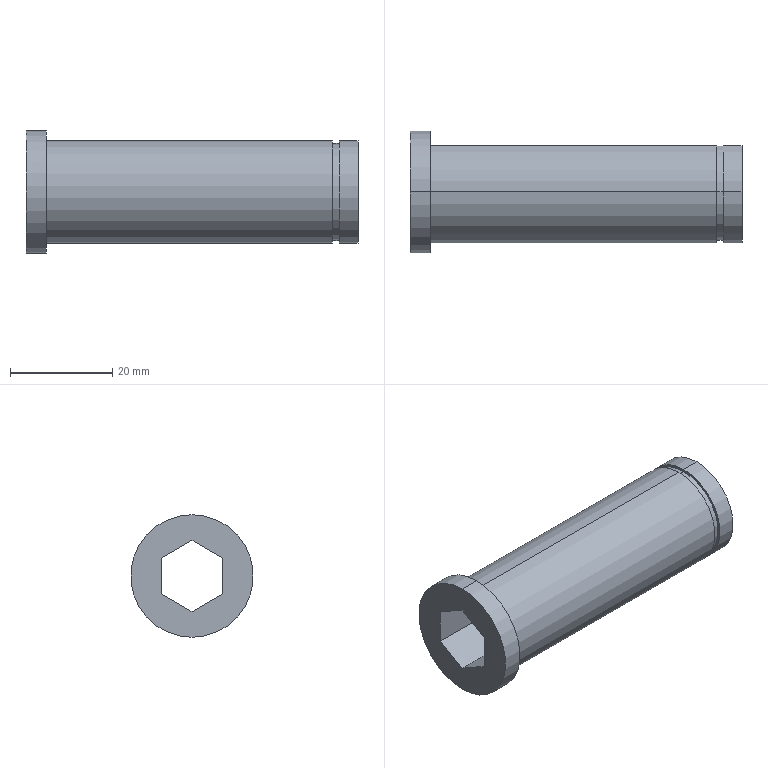Part | SolidWorks | features BaseBody 1 | 1 solid | 23 faces | box 65 x 24 x 24 mm | volume 12337 mm3 | plane 12 | cylinder 11 | commonest cylinder face diameters 20 x6 19 x3 24 x2
STEP:
#1=CARTESIAN_POINT('',(60.,9.,3.041));
#2=VERTEX_POINT('',#1);
#3=CARTESIAN_POINT('',(60.,0.,9.5));
#4=VERTEX_POINT('',#3);
#5=CARTESIAN_POINT('',(60.,0.,0.));
#6=DIRECTION('',(1.,0.,0.));
#7=DIRECTION('',(0.,0.,-1.));
#8=AXIS2_PLACEMENT_3D('',#5,#6,#7);
#9=CIRCLE('',#8,9.5);
#10=EDGE_CURVE('',#2,#4,#9,.T.);
#11=ORIENTED_EDGE('',*,*,#10,.T.);
#12=CARTESIAN_POINT('',(61.35,0.,9.5));
#13=VERTEX_POINT('',#12);
#14=CARTESIAN_POINT('',(65.,0.,9.5));
#15=DIRECTION('',(1.,0.,0.));
#16=VECTOR('',#15,1000.);
#17=LINE('',#14,#16);
#18=EDGE_CURVE('',#4,#13,#17,.T.);
#19=ORIENTED_EDGE('',*,*,#18,.T.);
#20=CARTESIAN_POINT('',(61.35,9.,3.041));
#21=VERTEX_POINT('',#20);
#22=CARTESIAN_POINT('',(61.35,0.,0.));
#23=DIRECTION('',(1.,0.,0.));
#24=DIRECTION('',(0.,0.,-1.));
#25=AXIS2_PLACEMENT_3D('',#22,#23,#24);
#26=CIRCLE('',#25,9.5);
#27=EDGE_CURVE('',#21,#13,#26,.T.);
#28=ORIENTED_EDGE('',*,*,#27,.F.);
#29=CARTESIAN_POINT('',(65.,9.,3.041));
#30=DIRECTION('',(-1.,0.,0.));
#31=VECTOR('',#30,1000.);
#32=LINE('',#29,#31);
#33=EDGE_CURVE('',#21,#2,#32,.T.);
#34=ORIENTED_EDGE('',*,*,#33,.T.);
#35=EDGE_LOOP('',(#11,#19,#28,#34));
#36=FACE_OUTER_BOUND('',#35,.T.);
#37=CARTESIAN_POINT('',(65.,0.,0.));
#38=DIRECTION('',(1.,0.,0.));
#39=DIRECTION('',(0.,0.,-1.));
#40=AXIS2_PLACEMENT_3D('',#37,#38,#39);
#41=CYLINDRICAL_SURFACE('',#40,9.5);
#42=ADVANCED_FACE('',(#36),#41,.T.);
#43=ORIENTED_EDGE('',*,*,#18,.F.);
#44=CARTESIAN_POINT('',(60.,0.,-9.5));
#45=VERTEX_POINT('',#44);
#46=CARTESIAN_POINT('',(60.,0.,0.));
#47=DIRECTION('',(1.,0.,0.));
#48=DIRECTION('',(0.,0.,-1.));
#49=AXIS2_PLACEMENT_3D('',#46,#47,#48);
#50=CIRCLE('',#49,9.5);
#51=EDGE_CURVE('',#4,#45,#50,.T.);
#52=ORIENTED_EDGE('',*,*,#51,.T.);
#53=CARTESIAN_POINT('',(61.35,0.,-9.5));
#54=VERTEX_POINT('',#53);
#55=CARTESIAN_POINT('',(65.,0.,-9.5));
#56=DIRECTION('',(1.,0.,0.));
#57=VECTOR('',#56,1000.);
#58=LINE('',#55,#57);
#59=EDGE_CURVE('',#45,#54,#58,.T.);
#60=ORIENTED_EDGE('',*,*,#59,.T.);
#61=CARTESIAN_POINT('',(61.35,0.,0.));
#62=DIRECTION('',(1.,0.,0.));
#63=DIRECTION('',(0.,0.,-1.));
#64=AXIS2_PLACEMENT_3D('',#61,#62,#63);
#65=CIRCLE('',#64,9.5);
#66=EDGE_CURVE('',#13,#54,#65,.T.);
#67=ORIENTED_EDGE('',*,*,#66,.F.);
#68=EDGE_LOOP('',(#43,#52,#60,#67));
#69=FACE_OUTER_BOUND('',#68,.T.);
#70=CARTESIAN_POINT('',(65.,0.,0.));
#71=DIRECTION('',(1.,0.,0.));
#72=DIRECTION('',(0.,0.,-1.));
#73=AXIS2_PLACEMENT_3D('',#70,#71,#72);
#74=CYLINDRICAL_SURFACE('',#73,9.5);
#75=ADVANCED_FACE('',(#69),#74,.T.);
#76=CARTESIAN_POINT('',(65.,0.,-10.));
#77=VERTEX_POINT('',#76);
#78=CARTESIAN_POINT('',(65.,9.,-4.359));
#79=VERTEX_POINT('',#78);
#80=CARTESIAN_POINT('',(65.,0.,0.));
#81=DIRECTION('',(1.,0.,0.));
#82=DIRECTION('',(0.,0.,-1.));
#83=AXIS2_PLACEMENT_3D('',#80,#81,#82);
#84=CIRCLE('',#83,10.);
#85=EDGE_CURVE('',#77,#79,#84,.T.);
#86=ORIENTED_EDGE('',*,*,#85,.F.);
#87=CARTESIAN_POINT('',(61.35,0.,-10.));
#88=VERTEX_POINT('',#87);
#89=CARTESIAN_POINT('',(77.,0.,-10.));
#90=DIRECTION('',(-1.,0.,0.));
#91=VECTOR('',#90,1000.);
#92=LINE('',#89,#91);
#93=EDGE_CURVE('',#77,#88,#92,.T.);
#94=ORIENTED_EDGE('',*,*,#93,.T.);
#95=CARTESIAN_POINT('',(61.35,9.,-4.359));
#96=VERTEX_POINT('',#95);
#97=CARTESIAN_POINT('',(61.35,0.,0.));
#98=DIRECTION('',(1.,0.,0.));
#99=DIRECTION('',(0.,0.,-1.));
#100=AXIS2_PLACEMENT_3D('',#97,#98,#99);
#101=CIRCLE('',#100,10.);
#102=EDGE_CURVE('',#88,#96,#101,.T.);
#103=ORIENTED_EDGE('',*,*,#102,.T.);
#104=CARTESIAN_POINT('',(77.,9.,-4.359));
#105=DIRECTION('',(1.,0.,0.));
#106=VECTOR('',#105,1000.);
#107=LINE('',#104,#106);
#108=EDGE_CURVE('',#96,#79,#107,.T.);
#109=ORIENTED_EDGE('',*,*,#108,.T.);
#110=EDGE_LOOP('',(#86,#94,#103,#109));
#111=FACE_OUTER_BOUND('',#110,.T.);
#112=CARTESIAN_POINT('',(77.,0.,0.));
#113=DIRECTION('',(-1.,0.,0.));
#114=DIRECTION('',(0.,0.,1.));
#115=AXIS2_PLACEMENT_3D('',#112,#113,#114);
#116=CYLINDRICAL_SURFACE('',#115,10.);
#117=ADVANCED_FACE('',(#111),#116,.T.);
#118=ORIENTED_EDGE('',*,*,#93,.F.);
#119=CARTESIAN_POINT('',(65.,0.,10.));
#120=VERTEX_POINT('',#119);
#121=CARTESIAN_POINT('',(65.,0.,0.));
#122=DIRECTION('',(1.,0.,0.));
#123=DIRECTION('',(0.,0.,-1.));
#124=AXIS2_PLACEMENT_3D('',#121,#122,#123);
#125=CIRCLE('',#124,10.);
#126=EDGE_CURVE('',#120,#77,#125,.T.);
#127=ORIENTED_EDGE('',*,*,#126,.F.);
#128=CARTESIAN_POINT('',(61.35,0.,10.));
#129=VERTEX_POINT('',#128);
#130=CARTESIAN_POINT('',(77.,0.,10.));
#131=DIRECTION('',(-1.,0.,0.));
#132=VECTOR('',#131,1000.);
#133=LINE('',#130,#132);
#134=EDGE_CURVE('',#120,#129,#133,.T.);
#135=ORIENTED_EDGE('',*,*,#134,.T.);
#136=CARTESIAN_POINT('',(61.35,0.,0.));
#137=DIRECTION('',(1.,0.,0.));
#138=DIRECTION('',(0.,0.,-1.));
#139=AXIS2_PLACEMENT_3D('',#136,#137,#138);
#140=CIRCLE('',#139,10.);
#141=EDGE_CURVE('',#129,#88,#140,.T.);
#142=ORIENTED_EDGE('',*,*,#141,.T.);
#143=EDGE_LOOP('',(#118,#127,#135,#142));
#144=FACE_OUTER_BOUND('',#143,.T.);
#145=CARTESIAN_POINT('',(77.,0.,0.));
#146=DIRECTION('',(-1.,0.,0.));
#147=DIRECTION('',(0.,0.,1.));
#148=AXIS2_PLACEMENT_3D('',#145,#146,#147);
#149=CYLINDRICAL_SURFACE('',#148,10.);
#150=ADVANCED_FACE('',(#144),#149,.T.);
#151=CARTESIAN_POINT('',(4.,0.,-12.));
#152=VERTEX_POINT('',#151);
#153=CARTESIAN_POINT('',(4.,0.,12.));
#154=VERTEX_POINT('',#153);
#155=CARTESIAN_POINT('',(4.,0.,0.));
#156=DIRECTION('',(1.,0.,0.));
#157=DIRECTION('',(0.,0.,-1.));
#158=AXIS2_PLACEMENT_3D('',#155,#156,#157);
#159=CIRCLE('',#158,12.);
#160=EDGE_CURVE('',#152,#154,#159,.T.);
#161=ORIENTED_EDGE('',*,*,#160,.F.);
#162=CARTESIAN_POINT('',(0.,0.,-12.));
#163=VERTEX_POINT('',#162);
#164=CARTESIAN_POINT('',(4.,0.,-12.));
#165=DIRECTION('',(-1.,0.,0.));
#166=VECTOR('',#165,1000.);
#167=LINE('',#164,#166);
#168=EDGE_CURVE('',#152,#163,#167,.T.);
#169=ORIENTED_EDGE('',*,*,#168,.T.);
#170=CARTESIAN_POINT('',(0.,0.,12.));
#171=VERTEX_POINT('',#170);
#172=CARTESIAN_POINT('',(0.,0.,0.));
#173=DIRECTION('',(1.,0.,0.));
#174=DIRECTION('',(0.,0.,-1.));
#175=AXIS2_PLACEMENT_3D('',#172,#173,#174);
#176=CIRCLE('',#175,12.);
#177=EDGE_CURVE('',#163,#171,#176,.T.);
#178=ORIENTED_EDGE('',*,*,#177,.T.);
#179=CARTESIAN_POINT('',(4.,0.,12.));
#180=DIRECTION('',(-1.,0.,0.));
#181=VECTOR('',#180,1000.);
#182=LINE('',#179,#181);
#183=EDGE_CURVE('',#154,#171,#182,.T.);
#184=ORIENTED_EDGE('',*,*,#183,.F.);
#185=EDGE_LOOP('',(#161,#169,#178,#184));
#186=FACE_OUTER_BOUND('',#185,.T.);
#187=CARTESIAN_POINT('',(4.,0.,0.));
#188=DIRECTION('',(-1.,0.,0.));
#189=DIRECTION('',(0.,0.,1.));
#190=AXIS2_PLACEMENT_3D('',#187,#188,#189);
#191=CYLINDRICAL_SURFACE('',#190,12.);
#192=ADVANCED_FACE('',(#186),#191,.T.);
#193=CARTESIAN_POINT('',(60.,0.,-10.));
#194=VERTEX_POINT('',#193);
#195=CARTESIAN_POINT('',(60.,9.,-4.359));
#196=VERTEX_POINT('',#195);
#197=CARTESIAN_POINT('',(60.,0.,0.));
#198=DIRECTION('',(1.,0.,0.));
#199=DIRECTION('',(0.,0.,-1.));
#200=AXIS2_PLACEMENT_3D('',#197,#198,#199);
#201=CIRCLE('',#200,10.);
#202=EDGE_CURVE('',#194,#196,#201,.T.);
#203=ORIENTED_EDGE('',*,*,#202,.F.);
#204=CARTESIAN_POINT('',(4.,0.,-10.));
#205=VERTEX_POINT('',#204);
#206=CARTESIAN_POINT('',(77.,0.,-10.));
#207=DIRECTION('',(-1.,0.,0.));
#208=VECTOR('',#207,1000.);
#209=LINE('',#206,#208);
#210=EDGE_CURVE('',#194,#205,#209,.T.);
#211=ORIENTED_EDGE('',*,*,#210,.T.);
#212=CARTESIAN_POINT('',(4.,9.,-4.359));
#213=VERTEX_POINT('',#212);
#214=CARTESIAN_POINT('',(4.,0.,0.));
#215=DIRECTION('',(1.,0.,0.));
#216=DIRECTION('',(0.,0.,-1.));
#217=AXIS2_PLACEMENT_3D('',#214,#215,#216);
#218=CIRCLE('',#217,10.);
#219=EDGE_CURVE('',#205,#213,#218,.T.);
#220=ORIENTED_EDGE('',*,*,#219,.T.);
#221=CARTESIAN_POINT('',(77.,9.,-4.359));
#222=DIRECTION('',(1.,0.,0.));
#223=VECTOR('',#222,1000.);
#224=LINE('',#221,#223);
#225=EDGE_CURVE('',#213,#196,#224,.T.);
#226=ORIENTED_EDGE('',*,*,#225,.T.);
#227=EDGE_LOOP('',(#203,#211,#220,#226));
#228=FACE_OUTER_BOUND('',#227,.T.);
#229=CARTESIAN_POINT('',(77.,0.,0.));
#230=DIRECTION('',(-1.,0.,0.));
#231=DIRECTION('',(0.,0.,1.));
#232=AXIS2_PLACEMENT_3D('',#229,#230,#231);
#233=CYLINDRICAL_SURFACE('',#232,10.);
#234=ADVANCED_FACE('',(#228),#233,.T.);
#235=ORIENTED_EDGE('',*,*,#210,.F.);
#236=CARTESIAN_POINT('',(60.,0.,10.));
#237=VERTEX_POINT('',#236);
#238=CARTESIAN_POINT('',(60.,0.,0.));
#239=DIRECTION('',(1.,0.,0.));
#240=DIRECTION('',(0.,0.,-1.));
#241=AXIS2_PLACEMENT_3D('',#238,#239,#240);
#242=CIRCLE('',#241,10.);
#243=EDGE_CURVE('',#237,#194,#242,.T.);
#244=ORIENTED_EDGE('',*,*,#243,.F.);
#245=CARTESIAN_POINT('',(4.,0.,10.));
#246=VERTEX_POINT('',#245);
#247=CARTESIAN_POINT('',(77.,0.,10.));
#248=DIRECTION('',(-1.,0.,0.));
#249=VECTOR('',#248,1000.);
#250=LINE('',#247,#249);
#251=EDGE_CURVE('',#237,#246,#250,.T.);
#252=ORIENTED_EDGE('',*,*,#251,.T.);
#253=CARTESIAN_POINT('',(4.,0.,0.));
#254=DIRECTION('',(1.,0.,0.));
#255=DIRECTION('',(0.,0.,-1.));
#256=AXIS2_PLACEMENT_3D('',#253,#254,#255);
#257=CIRCLE('',#256,10.);
#258=EDGE_CURVE('',#246,#205,#257,.T.);
#259=ORIENTED_EDGE('',*,*,#258,.T.);
#260=EDGE_LOOP('',(#235,#244,#252,#259));
#261=FACE_OUTER_BOUND('',#260,.T.);
#262=CARTESIAN_POINT('',(77.,0.,0.));
#263=DIRECTION('',(-1.,0.,0.));
#264=DIRECTION('',(0.,0.,1.));
#265=AXIS2_PLACEMENT_3D('',#262,#263,#264);
#266=CYLINDRICAL_SURFACE('',#265,10.);
#267=ADVANCED_FACE('',(#261),#266,.T.);
#268=CARTESIAN_POINT('',(0.,-6.05,-3.493));
#269=VERTEX_POINT('',#268);
#270=CARTESIAN_POINT('',(0.,-6.05,3.493));
#271=VERTEX_POINT('',#270);
#272=CARTESIAN_POINT('',(0.,-6.05,-3.493));
#273=DIRECTION('',(0.,0.,1.));
#274=VECTOR('',#273,1000.);
#275=LINE('',#272,#274);
#276=EDGE_CURVE('',#269,#271,#275,.T.);
#277=ORIENTED_EDGE('',*,*,#276,.T.);
#278=CARTESIAN_POINT('',(65.,-6.05,3.493));
#279=VERTEX_POINT('',#278);
#280=CARTESIAN_POINT('',(65.,-6.05,3.493));
#281=DIRECTION('',(-1.,0.,0.));
#282=VECTOR('',#281,1000.);
#283=LINE('',#280,#282);
#284=EDGE_CURVE('',#279,#271,#283,.T.);
#285=ORIENTED_EDGE('',*,*,#284,.F.);
#286=CARTESIAN_POINT('',(65.,-6.05,-3.493));
#287=VERTEX_POINT('',#286);
#288=CARTESIAN_POINT('',(65.,-6.05,-3.493));
#289=DIRECTION('',(0.,0.,1.));
#290=VECTOR('',#289,1000.);
#291=LINE('',#288,#290);
#292=EDGE_CURVE('',#287,#279,#291,.T.);
#293=ORIENTED_EDGE('',*,*,#292,.F.);
#294=CARTESIAN_POINT('',(65.,-6.05,-3.493));
#295=DIRECTION('',(-1.,0.,0.));
#296=VECTOR('',#295,1000.);
#297=LINE('',#294,#296);
#298=EDGE_CURVE('',#287,#269,#297,.T.);
#299=ORIENTED_EDGE('',*,*,#298,.T.);
#300=EDGE_LOOP('',(#277,#285,#293,#299));
#301=FACE_OUTER_BOUND('',#300,.T.);
#302=CARTESIAN_POINT('',(65.,-6.05,-3.493));
#303=DIRECTION('',(0.,-1.,0.));
#304=DIRECTION('',(0.,0.,-1.));
#305=AXIS2_PLACEMENT_3D('',#302,#303,#304);
#306=PLANE('',#305);
#307=ADVANCED_FACE('',(#301),#306,.F.);
#308=CARTESIAN_POINT('',(0.,0.,6.986));
#309=VERTEX_POINT('',#308);
#310=CARTESIAN_POINT('',(0.,-6.05,3.493));
#311=DIRECTION('',(0.,0.866,0.5));
#312=VECTOR('',#311,1000.);
#313=LINE('',#310,#312);
#314=EDGE_CURVE('',#271,#309,#313,.T.);
#315=ORIENTED_EDGE('',*,*,#314,.T.);
#316=CARTESIAN_POINT('',(65.,0.,6.986));
#317=VERTEX_POINT('',#316);
#318=CARTESIAN_POINT('',(65.,0.,6.986));
#319=DIRECTION('',(-1.,0.,0.));
#320=VECTOR('',#319,1000.);
#321=LINE('',#318,#320);
#322=EDGE_CURVE('',#317,#309,#321,.T.);
#323=ORIENTED_EDGE('',*,*,#322,.F.);
#324=CARTESIAN_POINT('',(65.,-6.05,3.493));
#325=DIRECTION('',(0.,0.866,0.5));
#326=VECTOR('',#325,1000.);
#327=LINE('',#324,#326);
#328=EDGE_CURVE('',#279,#317,#327,.T.);
#329=ORIENTED_EDGE('',*,*,#328,.F.);
#330=ORIENTED_EDGE('',*,*,#284,.T.);
#331=EDGE_LOOP('',(#315,#323,#329,#330));
#332=FACE_OUTER_BOUND('',#331,.T.);
#333=CARTESIAN_POINT('',(65.,-6.05,3.493));
#334=DIRECTION('',(0.,-0.5,0.866));
#335=DIRECTION('',(-1.,0.,0.));
#336=AXIS2_PLACEMENT_3D('',#333,#334,#335);
#337=PLANE('',#336);
#338=ADVANCED_FACE('',(#332),#337,.F.);
#339=CARTESIAN_POINT('',(0.,6.05,3.493));
#340=VERTEX_POINT('',#339);
#341=CARTESIAN_POINT('',(0.,0.,6.986));
#342=DIRECTION('',(0.,0.866,-0.5));
#343=VECTOR('',#342,1000.);
#344=LINE('',#341,#343);
#345=EDGE_CURVE('',#309,#340,#344,.T.);
#346=ORIENTED_EDGE('',*,*,#345,.T.);
#347=CARTESIAN_POINT('',(65.,6.05,3.493));
#348=VERTEX_POINT('',#347);
#349=CARTESIAN_POINT('',(65.,6.05,3.493));
#350=DIRECTION('',(-1.,0.,0.));
#351=VECTOR('',#350,1000.);
#352=LINE('',#349,#351);
#353=EDGE_CURVE('',#348,#340,#352,.T.);
#354=ORIENTED_EDGE('',*,*,#353,.F.);
#355=CARTESIAN_POINT('',(65.,0.,6.986));
#356=DIRECTION('',(0.,0.866,-0.5));
#357=VECTOR('',#356,1000.);
#358=LINE('',#355,#357);
#359=EDGE_CURVE('',#317,#348,#358,.T.);
#360=ORIENTED_EDGE('',*,*,#359,.F.);
#361=ORIENTED_EDGE('',*,*,#322,.T.);
#362=EDGE_LOOP('',(#346,#354,#360,#361));
#363=FACE_OUTER_BOUND('',#362,.T.);
#364=CARTESIAN_POINT('',(65.,0.,6.986));
#365=DIRECTION('',(0.,0.5,0.866));
#366=DIRECTION('',(1.,0.,0.));
#367=AXIS2_PLACEMENT_3D('',#364,#365,#366);
#368=PLANE('',#367);
#369=ADVANCED_FACE('',(#363),#368,.F.);
#370=CARTESIAN_POINT('',(0.,6.05,-3.493));
#371=VERTEX_POINT('',#370);
#372=CARTESIAN_POINT('',(0.,6.05,3.493));
#373=DIRECTION('',(0.,0.,-1.));
#374=VECTOR('',#373,1000.);
#375=LINE('',#372,#374);
#376=EDGE_CURVE('',#340,#371,#375,.T.);
#377=ORIENTED_EDGE('',*,*,#376,.T.);
#378=CARTESIAN_POINT('',(65.,6.05,-3.493));
#379=VERTEX_POINT('',#378);
#380=CARTESIAN_POINT('',(65.,6.05,-3.493));
#381=DIRECTION('',(-1.,0.,0.));
#382=VECTOR('',#381,1000.);
#383=LINE('',#380,#382);
#384=EDGE_CURVE('',#379,#371,#383,.T.);
#385=ORIENTED_EDGE('',*,*,#384,.F.);
#386=CARTESIAN_POINT('',(65.,6.05,3.493));
#387=DIRECTION('',(0.,0.,-1.));
#388=VECTOR('',#387,1000.);
#389=LINE('',#386,#388);
#390=EDGE_CURVE('',#348,#379,#389,.T.);
#391=ORIENTED_EDGE('',*,*,#390,.F.);
#392=ORIENTED_EDGE('',*,*,#353,.T.);
#393=EDGE_LOOP('',(#377,#385,#391,#392));
#394=FACE_OUTER_BOUND('',#393,.T.);
#395=CARTESIAN_POINT('',(65.,6.05,3.493));
#396=DIRECTION('',(0.,1.,0.));
#397=DIRECTION('',(1.,0.,0.));
#398=AXIS2_PLACEMENT_3D('',#395,#396,#397);
#399=PLANE('',#398);
#400=ADVANCED_FACE('',(#394),#399,.F.);
#401=CARTESIAN_POINT('',(0.,0.,-6.986));
#402=VERTEX_POINT('',#401);
#403=CARTESIAN_POINT('',(0.,6.05,-3.493));
#404=DIRECTION('',(0.,-0.866,-0.5));
#405=VECTOR('',#404,1000.);
#406=LINE('',#403,#405);
#407=EDGE_CURVE('',#371,#402,#406,.T.);
#408=ORIENTED_EDGE('',*,*,#407,.T.);
#409=CARTESIAN_POINT('',(65.,0.,-6.986));
#410=VERTEX_POINT('',#409);
#411=CARTESIAN_POINT('',(65.,0.,-6.986));
#412=DIRECTION('',(-1.,0.,0.));
#413=VECTOR('',#412,1000.);
#414=LINE('',#411,#413);
#415=EDGE_CURVE('',#410,#402,#414,.T.);
#416=ORIENTED_EDGE('',*,*,#415,.F.);
#417=CARTESIAN_POINT('',(65.,6.05,-3.493));
#418=DIRECTION('',(0.,-0.866,-0.5));
#419=VECTOR('',#418,1000.);
#420=LINE('',#417,#419);
#421=EDGE_CURVE('',#379,#410,#420,.T.);
#422=ORIENTED_EDGE('',*,*,#421,.F.);
#423=ORIENTED_EDGE('',*,*,#384,.T.);
#424=EDGE_LOOP('',(#408,#416,#422,#423));
#425=FACE_OUTER_BOUND('',#424,.T.);
#426=CARTESIAN_POINT('',(65.,6.05,-3.493));
#427=DIRECTION('',(0.,0.5,-0.866));
#428=DIRECTION('',(-1.,0.,0.));
#429=AXIS2_PLACEMENT_3D('',#426,#427,#428);
#430=PLANE('',#429);
#431=ADVANCED_FACE('',(#425),#430,.F.);
#432=CARTESIAN_POINT('',(0.,0.,-6.986));
#433=DIRECTION('',(0.,-0.866,0.5));
#434=VECTOR('',#433,1000.);
#435=LINE('',#432,#434);
#436=EDGE_CURVE('',#402,#269,#435,.T.);
#437=ORIENTED_EDGE('',*,*,#436,.T.);
#438=ORIENTED_EDGE('',*,*,#298,.F.);
#439=CARTESIAN_POINT('',(65.,0.,-6.986));
#440=DIRECTION('',(0.,-0.866,0.5));
#441=VECTOR('',#440,1000.);
#442=LINE('',#439,#441);
#443=EDGE_CURVE('',#410,#287,#442,.T.);
#444=ORIENTED_EDGE('',*,*,#443,.F.);
#445=ORIENTED_EDGE('',*,*,#415,.T.);
#446=EDGE_LOOP('',(#437,#438,#444,#445));
#447=FACE_OUTER_BOUND('',#446,.T.);
#448=CARTESIAN_POINT('',(65.,0.,-6.986));
#449=DIRECTION('',(0.,-0.5,-0.866));
#450=DIRECTION('',(0.,-0.866,0.5));
#451=AXIS2_PLACEMENT_3D('',#448,#449,#450);
#452=PLANE('',#451);
#453=ADVANCED_FACE('',(#447),#452,.F.);
#454=CARTESIAN_POINT('',(4.,9.,4.359));
#455=VERTEX_POINT('',#454);
#456=CARTESIAN_POINT('',(4.,9.,-25.));
#457=DIRECTION('',(0.,0.,1.));
#458=VECTOR('',#457,1000.);
#459=LINE('',#456,#458);
#460=EDGE_CURVE('',#213,#455,#459,.T.);
#461=ORIENTED_EDGE('',*,*,#460,.T.);
#462=CARTESIAN_POINT('',(60.,9.,4.359));
#463=VERTEX_POINT('',#462);
#464=CARTESIAN_POINT('',(77.,9.,4.359));
#465=DIRECTION('',(-1.,0.,0.));
#466=VECTOR('',#465,1000.);
#467=LINE('',#464,#466);
#468=EDGE_CURVE('',#463,#455,#467,.T.);
#469=ORIENTED_EDGE('',*,*,#468,.F.);
#470=CARTESIAN_POINT('',(60.,9.,0.));
#471=DIRECTION('',(0.,0.,1.));
#472=VECTOR('',#471,1000.);
#473=LINE('',#470,#472);
#474=EDGE_CURVE('',#2,#463,#473,.T.);
#475=ORIENTED_EDGE('',*,*,#474,.F.);
#476=ORIENTED_EDGE('',*,*,#33,.F.);
#477=CARTESIAN_POINT('',(61.35,9.,4.359));
#478=VERTEX_POINT('',#477);
#479=CARTESIAN_POINT('',(61.35,9.,0.));
#480=DIRECTION('',(0.,0.,-1.));
#481=VECTOR('',#480,1000.);
#482=LINE('',#479,#481);
#483=EDGE_CURVE('',#478,#21,#482,.T.);
#484=ORIENTED_EDGE('',*,*,#483,.F.);
#485=CARTESIAN_POINT('',(65.,9.,4.359));
#486=VERTEX_POINT('',#485);
#487=CARTESIAN_POINT('',(77.,9.,4.359));
#488=DIRECTION('',(-1.,0.,0.));
#489=VECTOR('',#488,1000.);
#490=LINE('',#487,#489);
#491=EDGE_CURVE('',#486,#478,#490,.T.);
#492=ORIENTED_EDGE('',*,*,#491,.F.);
#493=CARTESIAN_POINT('',(65.,9.,-25.));
#494=DIRECTION('',(0.,0.,1.));
#495=VECTOR('',#494,1000.);
#496=LINE('',#493,#495);
#497=EDGE_CURVE('',#79,#486,#496,.T.);
#498=ORIENTED_EDGE('',*,*,#497,.F.);
#499=ORIENTED_EDGE('',*,*,#108,.F.);
#500=CARTESIAN_POINT('',(61.35,9.,-3.041));
#501=VERTEX_POINT('',#500);
#502=CARTESIAN_POINT('',(61.35,9.,0.));
#503=DIRECTION('',(0.,0.,-1.));
#504=VECTOR('',#503,1000.);
#505=LINE('',#502,#504);
#506=EDGE_CURVE('',#501,#96,#505,.T.);
#507=ORIENTED_EDGE('',*,*,#506,.F.);
#508=CARTESIAN_POINT('',(60.,9.,-3.041));
#509=VERTEX_POINT('',#508);
#510=CARTESIAN_POINT('',(65.,9.,-3.041));
#511=DIRECTION('',(1.,0.,0.));
#512=VECTOR('',#511,1000.);
#513=LINE('',#510,#512);
#514=EDGE_CURVE('',#509,#501,#513,.T.);
#515=ORIENTED_EDGE('',*,*,#514,.F.);
#516=CARTESIAN_POINT('',(60.,9.,0.));
#517=DIRECTION('',(0.,0.,1.));
#518=VECTOR('',#517,1000.);
#519=LINE('',#516,#518);
#520=EDGE_CURVE('',#196,#509,#519,.T.);
#521=ORIENTED_EDGE('',*,*,#520,.F.);
#522=ORIENTED_EDGE('',*,*,#225,.F.);
#523=EDGE_LOOP('',(#461,#469,#475,#476,#484,#492,#498,#499,#507,#515,#521,#522));
#524=FACE_OUTER_BOUND('',#523,.T.);
#525=CARTESIAN_POINT('',(77.,9.,-25.));
#526=DIRECTION('',(0.,-1.,0.));
#527=DIRECTION('',(0.,0.,-1.));
#528=AXIS2_PLACEMENT_3D('',#525,#526,#527);
#529=PLANE('',#528);
#530=ADVANCED_FACE('',(#524),#529,.F.);
#531=CARTESIAN_POINT('',(61.35,0.,0.));
#532=DIRECTION('',(1.,0.,0.));
#533=DIRECTION('',(0.,0.,-1.));
#534=AXIS2_PLACEMENT_3D('',#531,#532,#533);
#535=CIRCLE('',#534,10.);
#536=EDGE_CURVE('',#478,#129,#535,.T.);
#537=ORIENTED_EDGE('',*,*,#536,.F.);
#538=ORIENTED_EDGE('',*,*,#483,.T.);
#539=ORIENTED_EDGE('',*,*,#27,.T.);
#540=ORIENTED_EDGE('',*,*,#66,.T.);
#541=CARTESIAN_POINT('',(61.35,0.,0.));
#542=DIRECTION('',(1.,0.,0.));
#543=DIRECTION('',(0.,0.,-1.));
#544=AXIS2_PLACEMENT_3D('',#541,#542,#543);
#545=CIRCLE('',#544,9.5);
#546=EDGE_CURVE('',#54,#501,#545,.T.);
#547=ORIENTED_EDGE('',*,*,#546,.T.);
#548=ORIENTED_EDGE('',*,*,#506,.T.);
#549=ORIENTED_EDGE('',*,*,#102,.F.);
#550=ORIENTED_EDGE('',*,*,#141,.F.);
#551=EDGE_LOOP('',(#537,#538,#539,#540,#547,#548,#549,#550));
#552=FACE_OUTER_BOUND('',#551,.T.);
#553=CARTESIAN_POINT('',(61.35,9.5,0.));
#554=DIRECTION('',(1.,0.,0.));
#555=DIRECTION('',(0.,1.,0.));
#556=AXIS2_PLACEMENT_3D('',#553,#554,#555);
#557=PLANE('',#556);
#558=ADVANCED_FACE('',(#552),#557,.F.);
#559=ORIENTED_EDGE('',*,*,#474,.T.);
#560=CARTESIAN_POINT('',(60.,0.,0.));
#561=DIRECTION('',(1.,0.,0.));
#562=DIRECTION('',(0.,0.,-1.));
#563=AXIS2_PLACEMENT_3D('',#560,#561,#562);
#564=CIRCLE('',#563,10.);
#565=EDGE_CURVE('',#463,#237,#564,.T.);
#566=ORIENTED_EDGE('',*,*,#565,.T.);
#567=ORIENTED_EDGE('',*,*,#243,.T.);
#568=ORIENTED_EDGE('',*,*,#202,.T.);
#569=ORIENTED_EDGE('',*,*,#520,.T.);
#570=CARTESIAN_POINT('',(60.,0.,0.));
#571=DIRECTION('',(1.,0.,0.));
#572=DIRECTION('',(0.,0.,-1.));
#573=AXIS2_PLACEMENT_3D('',#570,#571,#572);
#574=CIRCLE('',#573,9.5);
#575=EDGE_CURVE('',#45,#509,#574,.T.);
#576=ORIENTED_EDGE('',*,*,#575,.F.);
#577=ORIENTED_EDGE('',*,*,#51,.F.);
#578=ORIENTED_EDGE('',*,*,#10,.F.);
#579=EDGE_LOOP('',(#559,#566,#567,#568,#569,#576,#577,#578));
#580=FACE_OUTER_BOUND('',#579,.T.);
#581=CARTESIAN_POINT('',(60.,9.5,0.));
#582=DIRECTION('',(-1.,0.,0.));
#583=DIRECTION('',(0.,0.,1.));
#584=AXIS2_PLACEMENT_3D('',#581,#582,#583);
#585=PLANE('',#584);
#586=ADVANCED_FACE('',(#580),#585,.F.);
#587=ORIENTED_EDGE('',*,*,#443,.T.);
#588=ORIENTED_EDGE('',*,*,#292,.T.);
#589=ORIENTED_EDGE('',*,*,#328,.T.);
#590=ORIENTED_EDGE('',*,*,#359,.T.);
#591=ORIENTED_EDGE('',*,*,#390,.T.);
#592=ORIENTED_EDGE('',*,*,#421,.T.);
#593=EDGE_LOOP('',(#587,#588,#589,#590,#591,#592));
#594=FACE_BOUND('',#593,.T.);
#595=ORIENTED_EDGE('',*,*,#497,.T.);
#596=CARTESIAN_POINT('',(65.,0.,0.));
#597=DIRECTION('',(1.,0.,0.));
#598=DIRECTION('',(0.,0.,-1.));
#599=AXIS2_PLACEMENT_3D('',#596,#597,#598);
#600=CIRCLE('',#599,10.);
#601=EDGE_CURVE('',#486,#120,#600,.T.);
#602=ORIENTED_EDGE('',*,*,#601,.T.);
#603=ORIENTED_EDGE('',*,*,#126,.T.);
#604=ORIENTED_EDGE('',*,*,#85,.T.);
#605=EDGE_LOOP('',(#595,#602,#603,#604));
#606=FACE_OUTER_BOUND('',#605,.T.);
#607=CARTESIAN_POINT('',(65.,0.,0.));
#608=DIRECTION('',(1.,0.,0.));
#609=DIRECTION('',(0.,1.,0.));
#610=AXIS2_PLACEMENT_3D('',#607,#608,#609);
#611=PLANE('',#610);
#612=ADVANCED_FACE('',(#594,#606),#611,.T.);
#613=ORIENTED_EDGE('',*,*,#276,.F.);
#614=ORIENTED_EDGE('',*,*,#436,.F.);
#615=ORIENTED_EDGE('',*,*,#407,.F.);
#616=ORIENTED_EDGE('',*,*,#376,.F.);
#617=ORIENTED_EDGE('',*,*,#345,.F.);
#618=ORIENTED_EDGE('',*,*,#314,.F.);
#619=EDGE_LOOP('',(#613,#614,#615,#616,#617,#618));
#620=FACE_BOUND('',#619,.T.);
#621=CARTESIAN_POINT('',(0.,0.,0.));
#622=DIRECTION('',(1.,0.,0.));
#623=DIRECTION('',(0.,0.,-1.));
#624=AXIS2_PLACEMENT_3D('',#621,#622,#623);
#625=CIRCLE('',#624,12.);
#626=EDGE_CURVE('',#171,#163,#625,.T.);
#627=ORIENTED_EDGE('',*,*,#626,.F.);
#628=ORIENTED_EDGE('',*,*,#177,.F.);
#629=EDGE_LOOP('',(#627,#628));
#630=FACE_OUTER_BOUND('',#629,.T.);
#631=CARTESIAN_POINT('',(0.,0.,0.));
#632=DIRECTION('',(1.,0.,0.));
#633=DIRECTION('',(0.,1.,0.));
#634=AXIS2_PLACEMENT_3D('',#631,#632,#633);
#635=PLANE('',#634);
#636=ADVANCED_FACE('',(#620,#630),#635,.F.);
#637=CARTESIAN_POINT('',(4.,0.,0.));
#638=DIRECTION('',(1.,0.,0.));
#639=DIRECTION('',(0.,0.,-1.));
#640=AXIS2_PLACEMENT_3D('',#637,#638,#639);
#641=CIRCLE('',#640,10.);
#642=EDGE_CURVE('',#455,#246,#641,.T.);
#643=ORIENTED_EDGE('',*,*,#642,.F.);
#644=ORIENTED_EDGE('',*,*,#460,.F.);
#645=ORIENTED_EDGE('',*,*,#219,.F.);
#646=ORIENTED_EDGE('',*,*,#258,.F.);
#647=EDGE_LOOP('',(#643,#644,#645,#646));
#648=FACE_BOUND('',#647,.T.);
#649=CARTESIAN_POINT('',(4.,0.,0.));
#650=DIRECTION('',(1.,0.,0.));
#651=DIRECTION('',(0.,0.,-1.));
#652=AXIS2_PLACEMENT_3D('',#649,#650,#651);
#653=CIRCLE('',#652,12.);
#654=EDGE_CURVE('',#154,#152,#653,.T.);
#655=ORIENTED_EDGE('',*,*,#654,.T.);
#656=ORIENTED_EDGE('',*,*,#160,.T.);
#657=EDGE_LOOP('',(#655,#656));
#658=FACE_OUTER_BOUND('',#657,.T.);
#659=CARTESIAN_POINT('',(4.,0.,0.));
#660=DIRECTION('',(1.,0.,0.));
#661=DIRECTION('',(0.,1.,0.));
#662=AXIS2_PLACEMENT_3D('',#659,#660,#661);
#663=PLANE('',#662);
#664=ADVANCED_FACE('',(#648,#658),#663,.T.);
#665=ORIENTED_EDGE('',*,*,#251,.F.);
#666=ORIENTED_EDGE('',*,*,#565,.F.);
#667=ORIENTED_EDGE('',*,*,#468,.T.);
#668=ORIENTED_EDGE('',*,*,#642,.T.);
#669=EDGE_LOOP('',(#665,#666,#667,#668));
#670=FACE_OUTER_BOUND('',#669,.T.);
#671=CARTESIAN_POINT('',(77.,0.,0.));
#672=DIRECTION('',(-1.,0.,0.));
#673=DIRECTION('',(0.,0.,1.));
#674=AXIS2_PLACEMENT_3D('',#671,#672,#673);
#675=CYLINDRICAL_SURFACE('',#674,10.);
#676=ADVANCED_FACE('',(#670),#675,.T.);
#677=ORIENTED_EDGE('',*,*,#168,.F.);
#678=ORIENTED_EDGE('',*,*,#654,.F.);
#679=ORIENTED_EDGE('',*,*,#183,.T.);
#680=ORIENTED_EDGE('',*,*,#626,.T.);
#681=EDGE_LOOP('',(#677,#678,#679,#680));
#682=FACE_OUTER_BOUND('',#681,.T.);
#683=CARTESIAN_POINT('',(4.,0.,0.));
#684=DIRECTION('',(-1.,0.,0.));
#685=DIRECTION('',(0.,0.,1.));
#686=AXIS2_PLACEMENT_3D('',#683,#684,#685);
#687=CYLINDRICAL_SURFACE('',#686,12.);
#688=ADVANCED_FACE('',(#682),#687,.T.);
#689=ORIENTED_EDGE('',*,*,#134,.F.);
#690=ORIENTED_EDGE('',*,*,#601,.F.);
#691=ORIENTED_EDGE('',*,*,#491,.T.);
#692=ORIENTED_EDGE('',*,*,#536,.T.);
#693=EDGE_LOOP('',(#689,#690,#691,#692));
#694=FACE_OUTER_BOUND('',#693,.T.);
#695=CARTESIAN_POINT('',(77.,0.,0.));
#696=DIRECTION('',(-1.,0.,0.));
#697=DIRECTION('',(0.,0.,1.));
#698=AXIS2_PLACEMENT_3D('',#695,#696,#697);
#699=CYLINDRICAL_SURFACE('',#698,10.);
#700=ADVANCED_FACE('',(#694),#699,.T.);
#701=ORIENTED_EDGE('',*,*,#59,.F.);
#702=ORIENTED_EDGE('',*,*,#575,.T.);
#703=ORIENTED_EDGE('',*,*,#514,.T.);
#704=ORIENTED_EDGE('',*,*,#546,.F.);
#705=EDGE_LOOP('',(#701,#702,#703,#704));
#706=FACE_OUTER_BOUND('',#705,.T.);
#707=CARTESIAN_POINT('',(65.,0.,0.));
#708=DIRECTION('',(1.,0.,0.));
#709=DIRECTION('',(0.,0.,-1.));
#710=AXIS2_PLACEMENT_3D('',#707,#708,#709);
#711=CYLINDRICAL_SURFACE('',#710,9.5);
#712=ADVANCED_FACE('',(#706),#711,.T.);
#713=CLOSED_SHELL('',(#42,#75,#117,#150,#192,#234,#267,#307,#338,#369,#400,#431,#453,#530,#558,#586,#612,#636,#664,#676,#688,#700,#712));
#714=MANIFOLD_SOLID_BREP('',#713);
#715=CARTESIAN_POINT('',(0.,0.,0.));
#716=DIRECTION('',(0.,0.,1.));
#717=DIRECTION('',(1.,0.,0.));
#718=AXIS2_PLACEMENT_3D('',#715,#716,#717);
#719=(LENGTH_UNIT()NAMED_UNIT(*)SI_UNIT(.MILLI.,.METRE.));
#720=UNCERTAINTY_MEASURE_WITH_UNIT(LENGTH_MEASURE(0.00001),#719,'','');
#721=(NAMED_UNIT(*)PLANE_ANGLE_UNIT()SI_UNIT($,.RADIAN.));
#722=(NAMED_UNIT(*)SI_UNIT($,.STERADIAN.)SOLID_ANGLE_UNIT());
#723=(GEOMETRIC_REPRESENTATION_CONTEXT(3)GLOBAL_UNCERTAINTY_ASSIGNED_CONTEXT((#720))GLOBAL_UNIT_ASSIGNED_CONTEXT((#719,#721,#722))REPRESENTATION_CONTEXT('',''));
#724=ADVANCED_BREP_SHAPE_REPRESENTATION('',(#714,#718),#723);